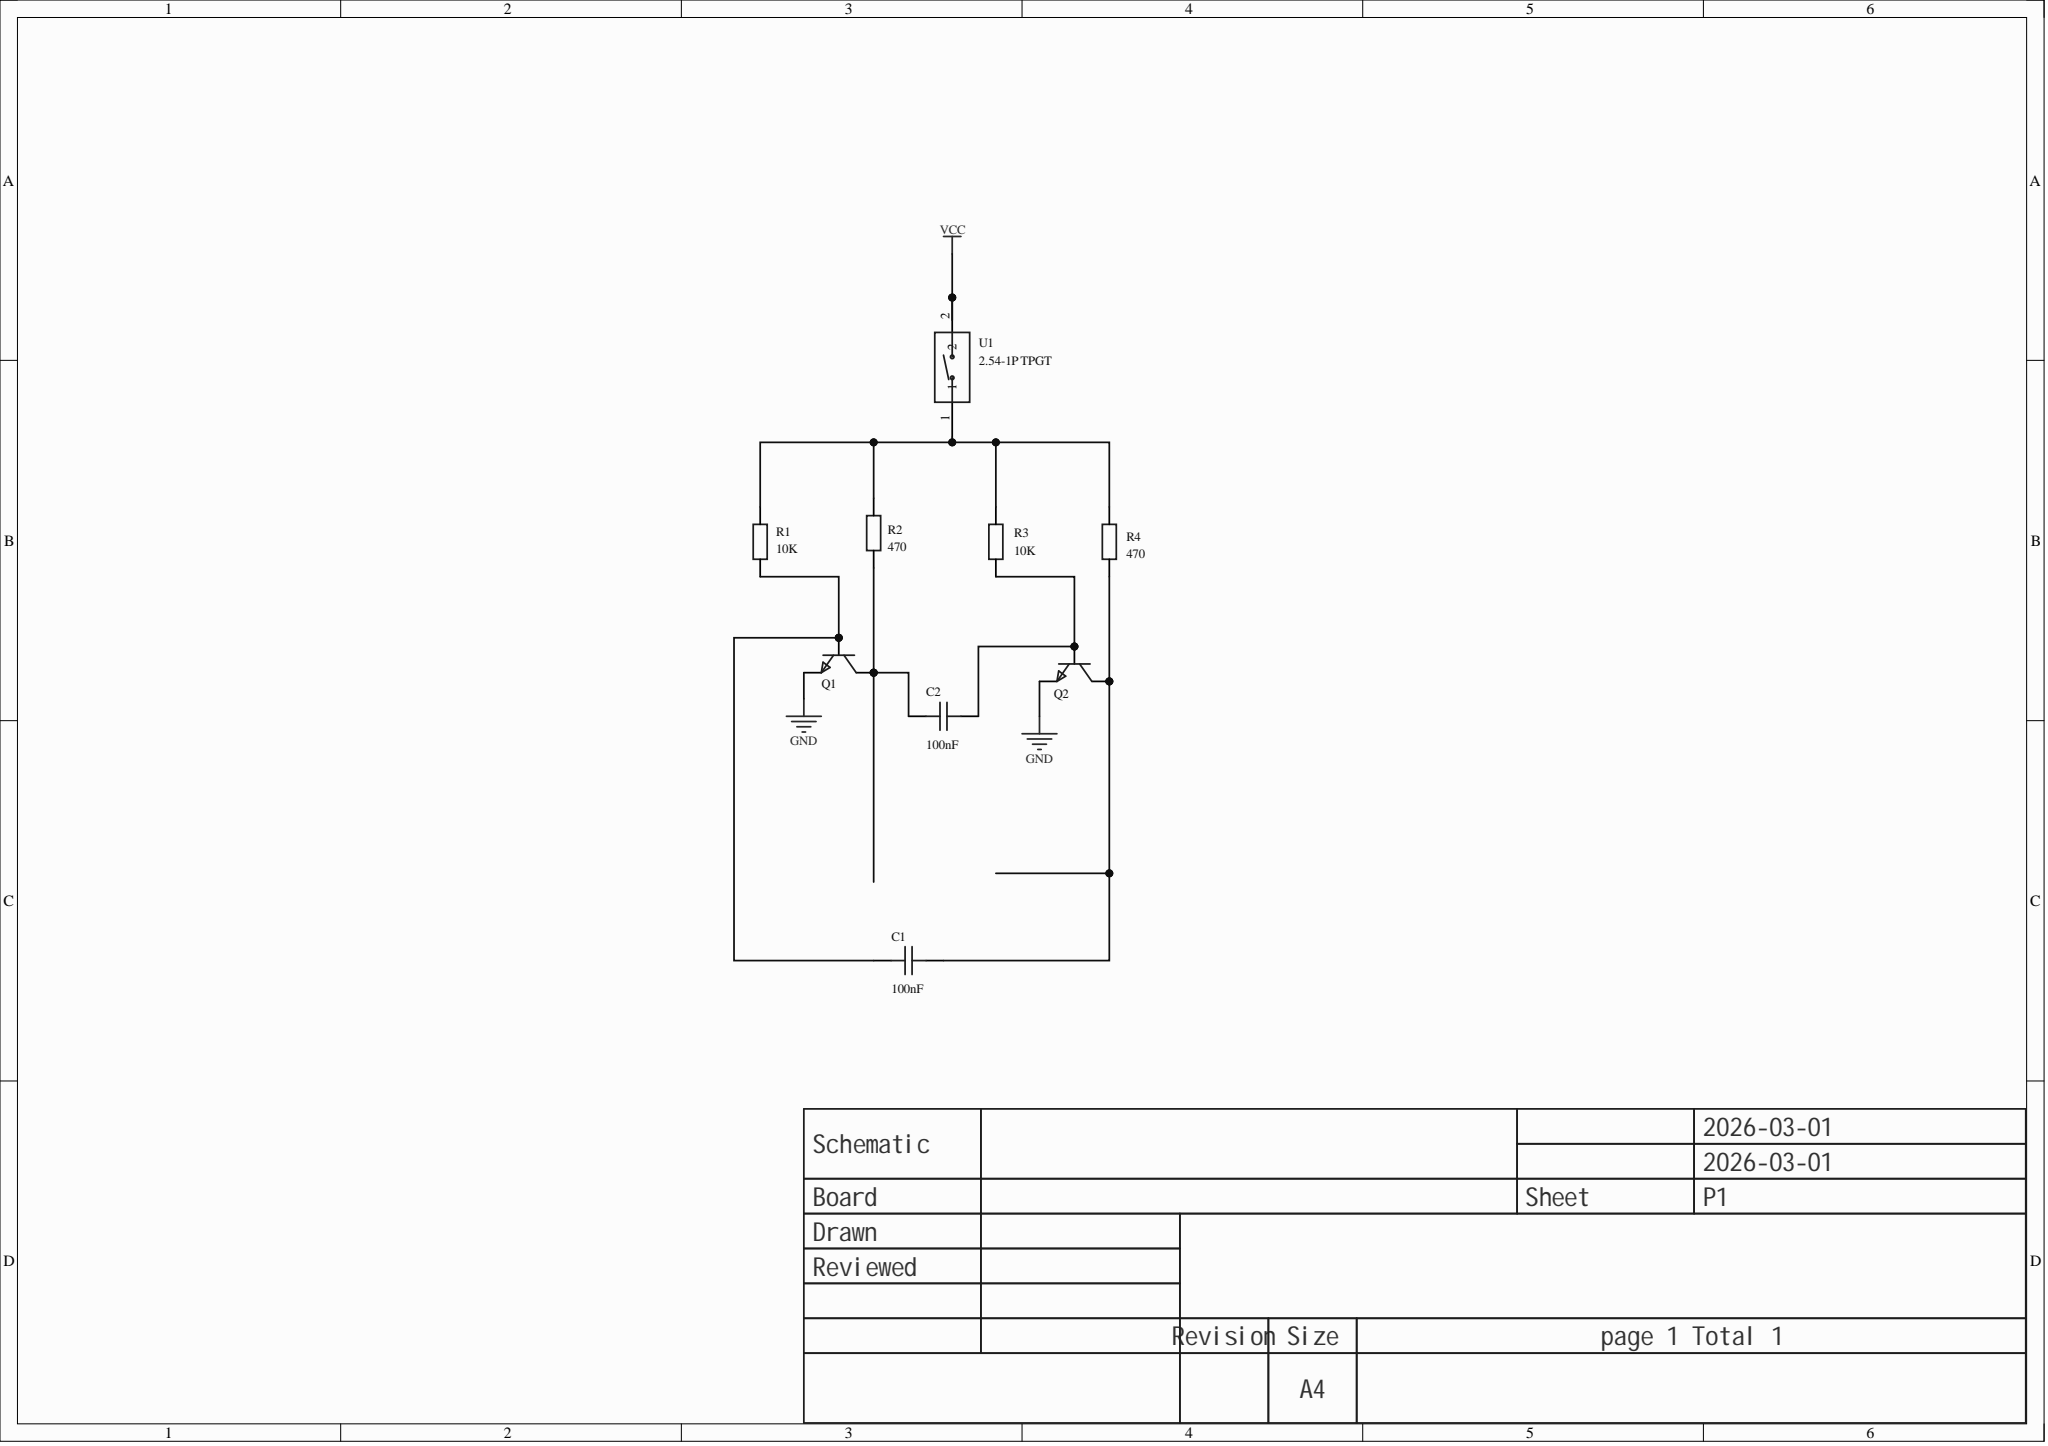Circuit board | Altium Designer | 9 parts | 6 nets
Bill of materials:
Comment,Description,Designator,Footprint,LibRef,Quantity
"100nF","","C1, C2","C0603","CAP_0603","2"
"","","Q1, Q2","S8050_SOT-23","S8050_SOT_NPN","2"
"10K","","R1, R3","R0603","Res_0603","2"
"470","","R2, R4","R0603","Res_0603","2"
"2.54-1P TPGT","","U1","SW-SMD_2P-L6.2-W2.5-LS9.4","2.54-1P TPGT","1"
Netlist (Protel format):
[
C1
C0603
100nF



]
[
C2
C0603
100nF



]
[
Q1
S8050_SOT-23




]
[
Q2
S8050_SOT-23




]
[
R1
R0603
10K



]
[
R2
R0603
470



]
[
R3
R0603
10K



]
[
R4
R0603
470



]
[
U1
SW-SMD_2P-L6.2-W2.5-LS9.4
2.54-1P TPGT



]
(
NetR1_2
R1-2
R2-2
R3-2
R4-2
U1-1
)
(
NetC2_2
C2-2
Q1-3
R2-1
)
(
NetC2_1
C2-1
Q2-1
R3-1
)
(
NetC1_2
C1-2
Q1-1
R1-1
)
(
NetC1_1
C1-1
Q2-3
R4-1
)
(
GND
Q1-2
Q2-2
)